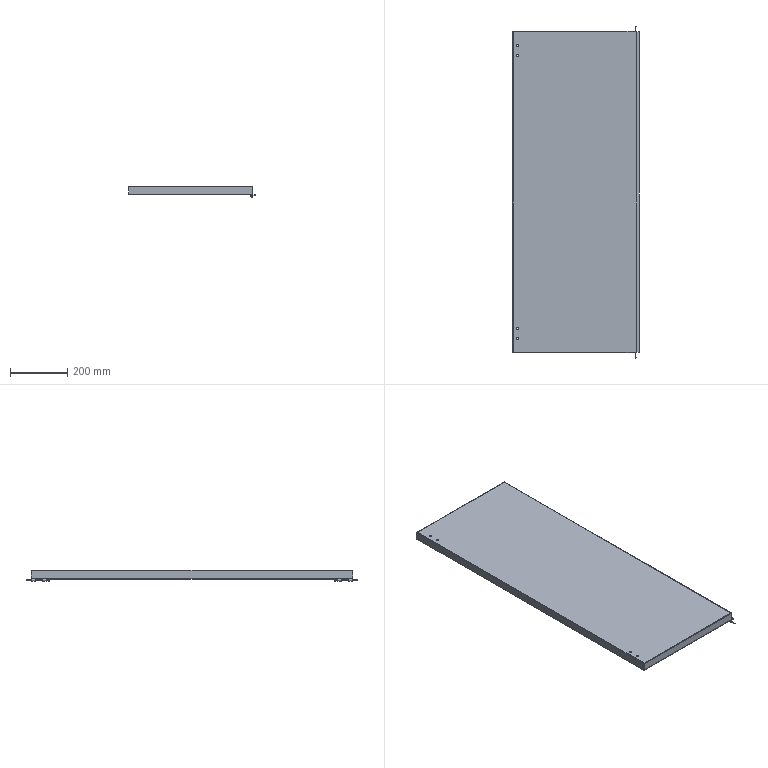Part | 5 solids | 145 faces | box 441.8 x 1156 x 41 mm | volume 727031 mm3 | plane 76 | cylinder 51 | spline 14 | torus 4 | commonest cylinder face diameters 7 x11 1.473 x8 3 x8 3.6 x8 3.873 x8 7.6 x8